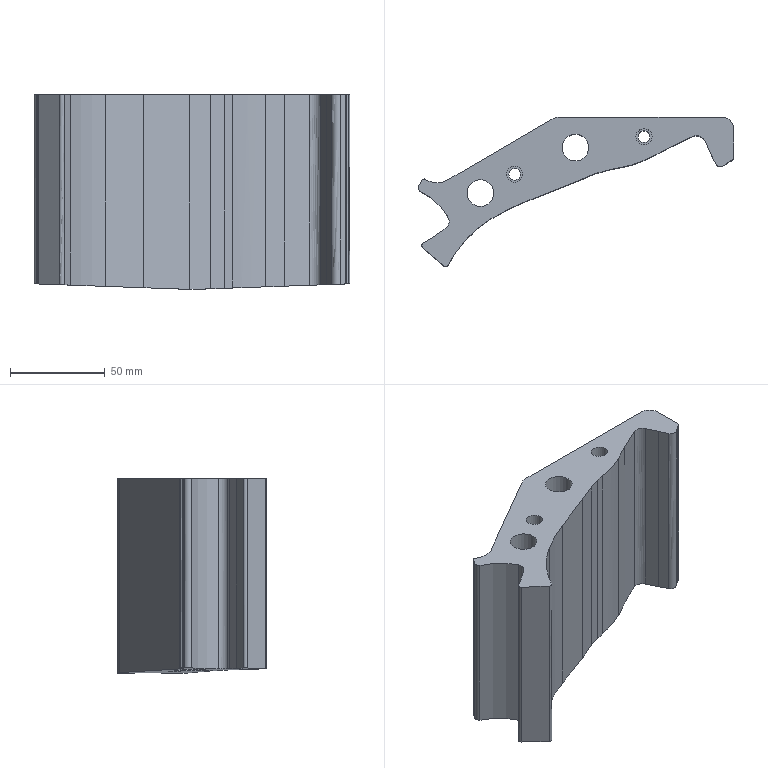Part | NX | features 8 2 | 1 solid | 56 faces | box 166.615 x 78.752 x 103 mm | volume 402781 mm3 | plane 23 | spline 23 | cylinder 10 | commonest cylinder face diameters 20 x3 6.2 x2 8.5 x2 14.1 x2 16 x1